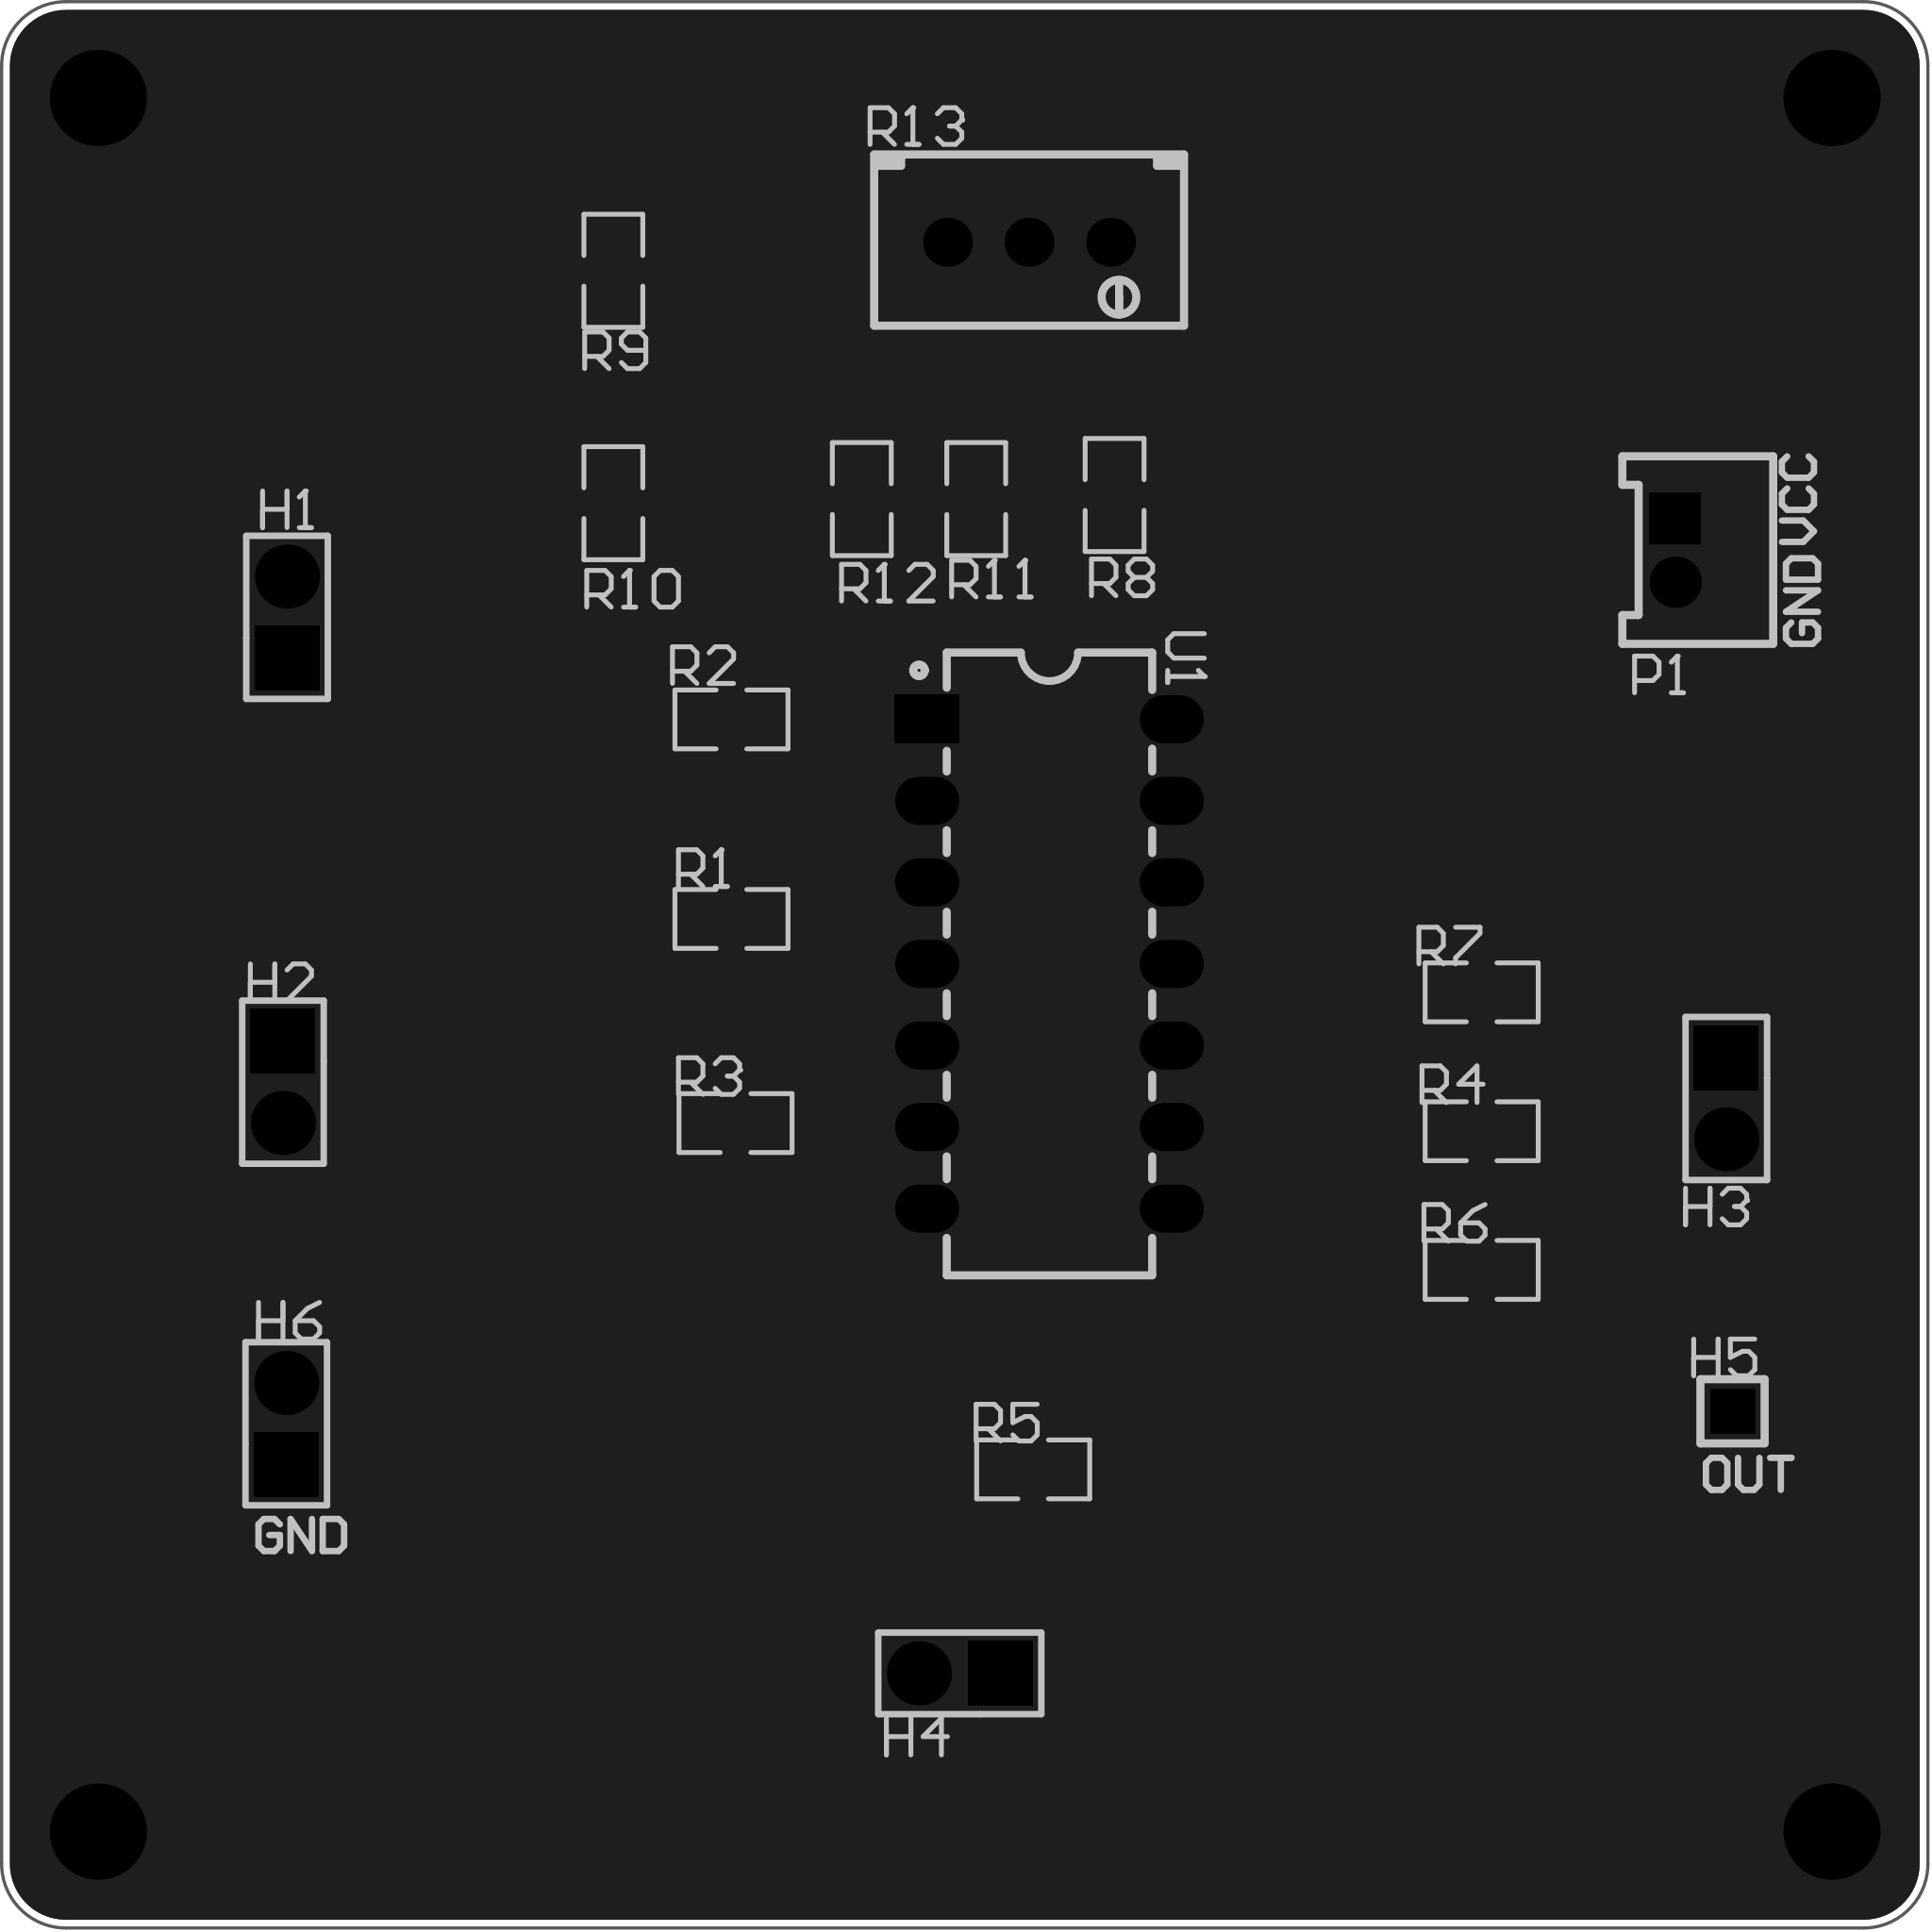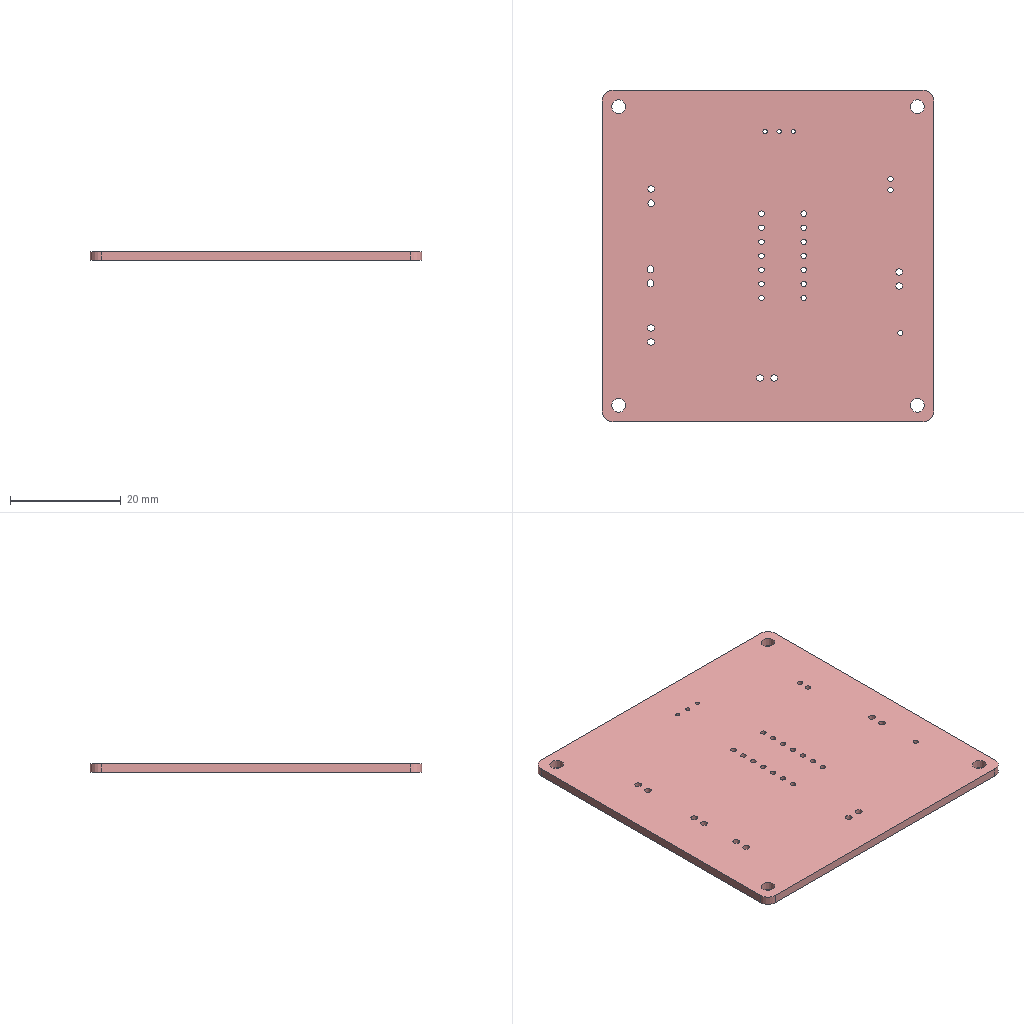Circuit board layout | Altium Designer | box 60 x 60 x 1.6 mm
Layer stack:
# Altium Designer layer stack of  (unit mm; dielectric type: 0 none, 1 core, 2 prepreg, 3 surface material)
index,name,kind,layer,copper_thickness_mm,dielectric_type,dielectric_thickness_mm,dielectric_material,dielectric_constant
0,Top Paste Mask Layer,other,,,,,,
1,Top Silkscreen Layer,other,,,,,,
2,Top Solder Mask Layer,dielectric,,,3,0.01,,3.3
3,Top Layer,copper,Top Layer,0.035,,,,
4,Dielectric1,dielectric,,,3,1.51,FR4,4.5
5,Bottom Layer,copper,Bottom Layer,0.035,,,,
6,Bottom Solder Mask Layer,dielectric,,,3,0.01,,3.3
7,Bottom Silkscreen Layer,other,,,,,,
8,Bottom Paste Mask Layer,other,,,,,,
# drill layer pairs: low layer,high layer
drill_pair,Top Layer,Bottom Layer
Part placement:
Designator,Comment,Layer,Footprint,Center-X(mm),Center-Y(mm),Rotation
H5,,TopLayer,HDR-TH_1P-V-M_XKB_X4611WV-01I-C28D40,137.226,97.063,270
P1,PH-2A,TopLayer,CONN-TH_2P-P2.00_PH-2A_C2319,135.446,123.888,90
R1,2K,TopLayer,R0805_1,106.045,112.395,180
R2,5K,TopLayer,R0805_1,106.045,118.618,0
R3,5K,TopLayer,R0805_1,106.172,106.045,0
R4,2K,TopLayer,R0805_1,129.413,105.791,0
R5,2K,TopLayer,R0805_1,115.443,95.25,180
R6,40K,TopLayer,R0805_1,129.413,101.473,0
R7,40K,TopLayer,R0805_1,129.413,110.109,180
R8,10K,TopLayer,R0805_1,117.983,125.603,270
R9,9.76K,TopLayer,R0805_1,102.362,132.588,90
R10,140,TopLayer,R0805_1,102.362,125.349,90
R11,10K,TopLayer,R0805_1,113.665,125.476,90
R12,10K,TopLayer,R0805_1,110.109,125.476,270
R13,100Ω,TopLayer,RES-ADJ-TH_3296W,115.316,133.477,270
U1,LM324N,TopLayer,DIP-14_L19.4-W6.4-P2.54-LS7.6-BL,115.951,110.998,270
H1,PZ254V-11-02P,TopLayer,HDR-TH_2P-P2.54-V-M,92.202,121.793,90
H2,PZ254V-11-02P,TopLayer,HDR-TH_2P-P2.54-V-M,92.075,107.315,270
H3,PZ254V-11-02P,TopLayer,HDR-TH_2P-P2.54-V-M,137.033,106.807,270
H4,PZ254V-11-02P,TopLayer,HDR-TH_2P-P2.54-V-M,113.157,88.9,180
H6,PZ254V-11-02P,TopLayer,HDR-TH_2P-P2.54-V-M,92.178,96.675,90
Pad and via stacks:
# Altium Designer via and pad stacks of  (unit mm). Each distinct definition once, with the count of objects using it.
# via: kind,start_layer,end_layer,hole_mm,diameter_mm,mode(0 simple;1 top-mid-bottom;2 full stack),diameter_per_layer,count,example_net
# pad: kind,layer,hole_mm,hole_type(0 round;1 square;2 slot),plating,top_size,top_shape(1 round;2 rect;3 octagon;9 rounded rect),mid_size,bottom_size,mode,footprint,size_per_layer,count,example
pad,Multi-Layer,0.9,0,plated,1.4x1.4,2,1.4x1.4,1.4x1.4,0,HDR-TH_1P-V-M_XKB_X4611WV-01I-C28D40,,1,H5.1
pad,Multi-Layer,1,0,plated,1.6x1.6,2,1.6x1.6,1.6x1.6,0,CONN-TH_2P-P2.00_PH-2A_C2319,,1,P1.1
pad,Multi-Layer,1,0,plated,1.6x1.6,1,1.6x1.6,1.6x1.6,0,CONN-TH_2P-P2.00_PH-2A_C2319,,1,P1.2
pad,Multi-Layer,0.762,0,plated,1.524x1.524,1,1.524x1.524,1.524x1.524,0,RES-ADJ-TH_3296W,,3,R13.2
pad,Multi-Layer,1,0,plated,2x1.5,1,2x1.5,2x1.5,0,DIP-14_L19.4-W6.4-P2.54-LS7.6-BL,,13,U1.8
pad,Multi-Layer,1,0,plated,2x1.5,2,2x1.5,2x1.5,0,DIP-14_L19.4-W6.4-P2.54-LS7.6-BL,,1,U1.1
pad,Multi-Layer,1.2,0,plated,2x2,2,2x2,2x2,0,HDR-TH_2P-P2.54-V-M,,5,H1.1
pad,Multi-Layer,1.2,0,plated,2x2,1,2x2,2x2,0,HDR-TH_2P-P2.54-V-M,,5,H1.2
pad,Multi-Layer,2.5,0,plated,3x3,1,3x3,3x3,0,,,4,4
pad,Top Layer,0,0,plated,1.133x1.377,2,1.133x1.377,1.133x1.377,0,R0805_1,,24,R1.1
Copper pours:
name,layer,net,type(0 solid;1 hatched;2 none)
Top Layer-GND,Top Layer,GND,0
Bottom Layer-GND,Bottom Layer,GND,0